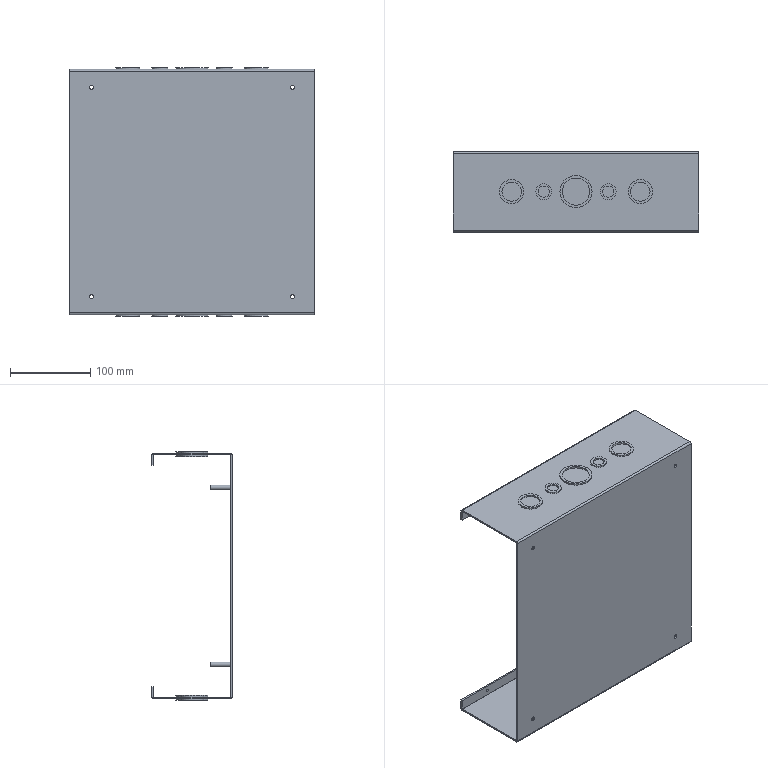Part | SolidWorks | features ICE 7, EdgeFlange 2, Cut 1, Fillet 1, FlatPattern 1, LPattern 1, SMBaseFlange 1, SheetMetal 1 | 1 solid | 186 faces | box 304.8 x 99.6 x 308.8 mm | volume 331493 mm3 | cylinder 112 | plane 74 | commonest cylinder face diameters 14 x16 20 x16 24 x16 30 x16 4 x8 5 x8